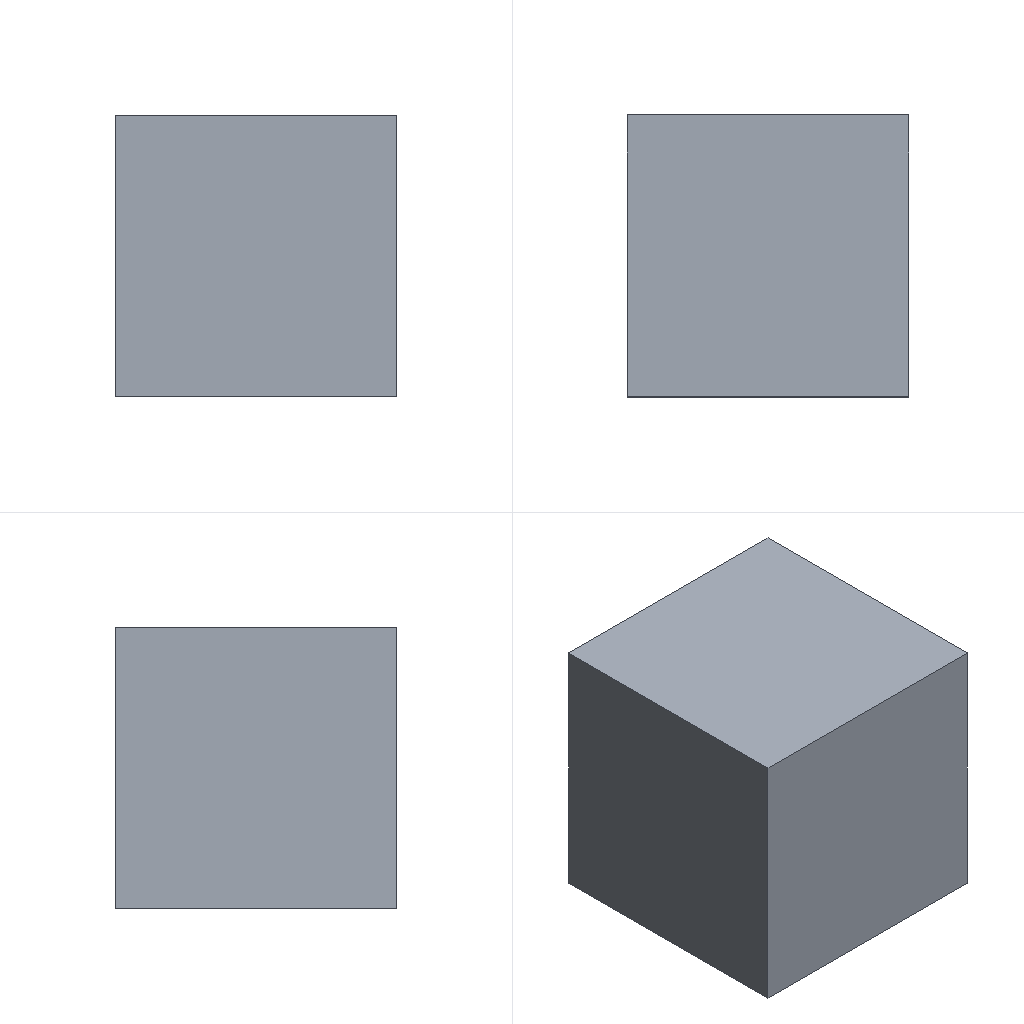Simulation study | abaqus
Set-up summary:
category,name,step,type,value,unit,region
solver,abaqus,,Abaqus/CAE 2024
units,unstated,,unstated
analysis,geostatic,,geostatic
analysis,load,,static,time_period=1
analysis,unload,,static,time_period=1
analysis,reload,,static,time_period=1
mesh,nodes,,,8
mesh,elements,,,1
element_type,C3D8,,,1
material,Material-1,,behaviors,depvar; user material
section,Material-1,,solid section,,,_PickedSet2
load,stress,initial,initial condition stress
load,,initial,initial condition solution
load,Load-1,geostatic,pressure,100,,_PickedSurf10
load,Load-2,load,pressure,200,,_PickedSurf6
load,Load-2,unload,pressure,100,,_PickedSurf6
load,Load-2,reload,pressure,300,,_PickedSurf6
bc,BC-1,initial,fixed,[dofs=z],,_PickedSet4
bc,BC-2,initial,fixed,[dofs=x],,_PickedSet8
bc,BC-3,initial,fixed,[dofs=y],,_PickedSet9
Abaqus input file, long lists of numbers shortened:
*Heading
** Job name: deck Model name: Model-1
** Generated by: Abaqus/CAE 2024
*Preprint, echo=NO, model=NO, history=NO, contact=NO
**
** PARTS
**
*Part, name=Part-1
*Node
      1,           1.,           1.,           1.
      2,           1.,           0.,           1.
** (6 more lines like these left out)
*Element, type=C3D8
1, 5, 6, 8, 7, 1, 2, 4, 3
*Nset, nset=_PickedSet2, internal, generate
 1,  8,  1
*Elset, elset=_PickedSet2, internal
 1,
*Nset, nset=soil, generate
 1,  8,  1
*Elset, elset=soil
 1,
** Section: Section-1
*Solid Section, elset=_PickedSet2, material=Material-1
1.,
*End Part
**
**
** ASSEMBLY
**
*Assembly, name=Assembly
**
*Instance, name=Part-1-1, part=Part-1
*End Instance
**
*Nset, nset=_PickedSet4, internal, instance=Part-1-1
 3, 4, 7, 8
*Elset, elset=_PickedSet4, internal, instance=Part-1-1
 1,
*Nset, nset=_PickedSet7, internal, instance=Part-1-1, generate
 1,  8,  1
*Elset, elset=_PickedSet7, internal, instance=Part-1-1
 1,
*Nset, nset=_PickedSet8, internal, instance=Part-1-1, generate
 5,  8,  1
*Elset, elset=_PickedSet8, internal, instance=Part-1-1
 1,
*Nset, nset=_PickedSet9, internal, instance=Part-1-1, generate
 2,  8,  2
*Elset, elset=_PickedSet9, internal, instance=Part-1-1
 1,
*Elset, elset=__PickedSurf6_S3, internal, instance=Part-1-1
 1,
*Surface, type=ELEMENT, name=_PickedSurf6, internal
__PickedSurf6_S3, S3
*Elset, elset=__PickedSurf10_S6, internal, instance=Part-1-1
 1,
*Elset, elset=__PickedSurf10_S2, internal, instance=Part-1-1
 1,
*Elset, elset=__PickedSurf10_S3, internal, instance=Part-1-1
 1,
*Surface, type=ELEMENT, name=_PickedSurf10, internal
__PickedSurf10_S6, S6
__PickedSurf10_S2, S2
__PickedSurf10_S3, S3
*End Assembly
**
** MATERIALS
**
*Material, name=Material-1
*Depvar
      3,
*User Material, constants=11
1000.,  0.5,  0.8,  10.,  30.,  0.3,   0.,   0.
1500., 100.,   0.
**
** BOUNDARY CONDITIONS
**
** Name: BC-1 Type: Displacement/Rotation
*Boundary
_PickedSet4, 3, 3
** Name: BC-2 Type: Displacement/Rotation
*Boundary
_PickedSet8, 1, 1
** Name: BC-3 Type: Displacement/Rotation
*Boundary
_PickedSet9, 2, 2
**
** PREDEFINED FIELDS
**
** Name: stress   Type: Stress
*Initial Conditions, type=STRESS
_PickedSet7, -100., -100., -100., 0., 0., 0.
*initial conditions,type=solution
part-1-1.soil,0,100,0
** ----------------------------------------------------------------
**
** STEP: geostatic
**
*Step, name=geostatic, nlgeom=NO
*Geostatic
**
** LOADS
**
** Name: Load-1   Type: Pressure
*Dsload
_PickedSurf10, P, 100.
**
** OUTPUT REQUESTS
**
*Restart, write, frequency=0
*Print, solve=NO
**
** FIELD OUTPUT: F-Output-1
**
*Output, field
*Node Output
CF, POR, RF, U
*Element Output, directions=YES
LE, S, SAT, SDV, VOIDR
*Contact Output
CDISP, CSTRESS
**
** HISTORY OUTPUT: H-Output-1
**
*Output, history, variable=PRESELECT
*End Step
** ----------------------------------------------------------------
**
** STEP: load
**
*Step, name=load, nlgeom=NO
*Static
0.01, 1., 1e-05, 0.01
**
** LOADS
**
** Name: Load-2   Type: Pressure
*Dsload
_PickedSurf6, P, 200.
**
** OUTPUT REQUESTS
**
*Restart, write, frequency=0
**
** FIELD OUTPUT: F-Output-1
**
*Output, field
*Node Output
CF, RF, U
*Element Output, directions=YES
LE, S, SDV
*Contact Output
CDISP, CSTRESS
**
** HISTORY OUTPUT: H-Output-1
**
*Output, history, variable=PRESELECT
*End Step
** ----------------------------------------------------------------
**
** STEP: unload
**
*Step, name=unload, nlgeom=NO, inc=1000
*Static
0.01, 1., 1e-05, 0.01
**
** LOADS
**
** Name: Load-2   Type: Pressure
*Dsload
_PickedSurf6, P, 100.
**
** OUTPUT REQUESTS
**
*Restart, write, frequency=0
**
** FIELD OUTPUT: F-Output-1
**
*Output, field
*Node Output
CF, RF, U
*Element Output, directions=YES
LE, S, SDV
*Contact Output
CDISP, CSTRESS
**
** HISTORY OUTPUT: H-Output-1
**
*Output, history, variable=PRESELECT
*End Step
** ----------------------------------------------------------------
**
** STEP: reload
**
*Step, name=reload, nlgeom=NO
*Static
0.01, 1., 1e-05, 0.01
**
** LOADS
**
** Name: Load-2   Type: Pressure
*Dsload
_PickedSurf6, P, 300.
**
** OUTPUT REQUESTS
**
*Restart, write, frequency=0
**
** FIELD OUTPUT: F-Output-1
**
*Output, field
*Node Output
CF, RF, U
*Element Output, directions=YES
LE, S, SDV
*Contact Output
CDISP, CSTRESS
**
** HISTORY OUTPUT: H-Output-1
**
*Output, history, variable=PRESELECT
*End Step
Results summary:
result,odb.job_status,,,JOB_STATUS_COMPLETED_SUCCESSFULLY,"consistent, unstated (Abaqus has no unit system)"
result,steps[0].procedure,geostatic,,*GEOSTATIC,"consistent, unstated (Abaqus has no unit system)"
result,steps[0].time_period,geostatic,,1,"consistent, unstated (Abaqus has no unit system)"
result,steps[0].n_frames,geostatic,,2,"consistent, unstated (Abaqus has no unit system)"
result,steps[0].last_frame.id,geostatic,,1,"consistent, unstated (Abaqus has no unit system)"
result,steps[0].last_frame.value,geostatic,,1,"consistent, unstated (Abaqus has no unit system)"
result,steps[0].last_frame.description,geostatic,,Increment      1: Step Time =    1.000,"consistent, unstated (Abaqus has no unit system)"
result,steps[0].completed,geostatic,,True,"consistent, unstated (Abaqus has no unit system)"
result,steps[0].max_U_magnitude,geostatic,,8.72122e-19,"consistent, unstated (Abaqus has no unit system)"
result,steps[0].max_S_mises,geostatic,,4.71813e-14,"consistent, unstated (Abaqus has no unit system)"
result,steps[0].RF_sum[1],geostatic,,100,"consistent, unstated (Abaqus has no unit system)"
result,steps[0].RF_sum[2],geostatic,,100,"consistent, unstated (Abaqus has no unit system)"
result,steps[0].RF_sum[3],geostatic,,100,"consistent, unstated (Abaqus has no unit system)"
result,steps[1].procedure,load,,*STATIC,"consistent, unstated (Abaqus has no unit system)"
result,steps[1].time_period,load,,1,"consistent, unstated (Abaqus has no unit system)"
result,steps[1].n_frames,load,,101,"consistent, unstated (Abaqus has no unit system)"
result,steps[1].last_frame.id,load,,100,"consistent, unstated (Abaqus has no unit system)"
result,steps[1].last_frame.value,load,,1,"consistent, unstated (Abaqus has no unit system)"
result,steps[1].last_frame.description,load,,Increment    100: Step Time =    1.000,"consistent, unstated (Abaqus has no unit system)"
result,steps[1].completed,load,,True,"consistent, unstated (Abaqus has no unit system)"
result,steps[1].max_U_magnitude,load,,0.006734,"consistent, unstated (Abaqus has no unit system)"
result,steps[1].max_S_mises,load,,200.003,"consistent, unstated (Abaqus has no unit system)"
result,steps[1].RF_sum[1],load,,100,"consistent, unstated (Abaqus has no unit system)"
result,steps[1].RF_sum[2],load,,100,"consistent, unstated (Abaqus has no unit system)"
result,steps[1].RF_sum[3],load,,300.003,"consistent, unstated (Abaqus has no unit system)"
result,steps[2].procedure,unload,,*STATIC,"consistent, unstated (Abaqus has no unit system)"
result,steps[2].time_period,unload,,1,"consistent, unstated (Abaqus has no unit system)"
result,steps[2].n_frames,unload,,103,"consistent, unstated (Abaqus has no unit system)"
result,steps[2].last_frame.id,unload,,102,"consistent, unstated (Abaqus has no unit system)"
result,steps[2].last_frame.value,unload,,1,"consistent, unstated (Abaqus has no unit system)"
result,steps[2].last_frame.description,unload,,Increment    102: Step Time =    1.000,"consistent, unstated (Abaqus has no unit system)"
result,steps[2].completed,unload,,True,"consistent, unstated (Abaqus has no unit system)"
result,steps[2].max_U_magnitude,unload,,0.00591,"consistent, unstated (Abaqus has no unit system)"
result,steps[2].max_S_mises,unload,,100,"consistent, unstated (Abaqus has no unit system)"
result,steps[2].RF_sum[1],unload,,100,"consistent, unstated (Abaqus has no unit system)"
result,steps[2].RF_sum[2],unload,,100,"consistent, unstated (Abaqus has no unit system)"
result,steps[2].RF_sum[3],unload,,200,"consistent, unstated (Abaqus has no unit system)"
result,steps[3].procedure,reload,,*STATIC,"consistent, unstated (Abaqus has no unit system)"
result,steps[3].time_period,reload,,1,"consistent, unstated (Abaqus has no unit system)"
result,steps[3].n_frames,reload,,101,"consistent, unstated (Abaqus has no unit system)"
result,steps[3].last_frame.id,reload,,100,"consistent, unstated (Abaqus has no unit system)"
result,steps[3].last_frame.value,reload,,1,"consistent, unstated (Abaqus has no unit system)"
result,steps[3].last_frame.description,reload,,Increment    100: Step Time =    1.000,"consistent, unstated (Abaqus has no unit system)"
result,steps[3].completed,reload,,True,"consistent, unstated (Abaqus has no unit system)"
result,steps[3].max_U_magnitude,reload,,0.02859,"consistent, unstated (Abaqus has no unit system)"
result,steps[3].max_S_mises,reload,,300,"consistent, unstated (Abaqus has no unit system)"
result,steps[3].RF_sum[1],reload,,100,"consistent, unstated (Abaqus has no unit system)"
result,steps[3].RF_sum[2],reload,,100,"consistent, unstated (Abaqus has no unit system)"
result,steps[3].RF_sum[3],reload,,400,"consistent, unstated (Abaqus has no unit system)"